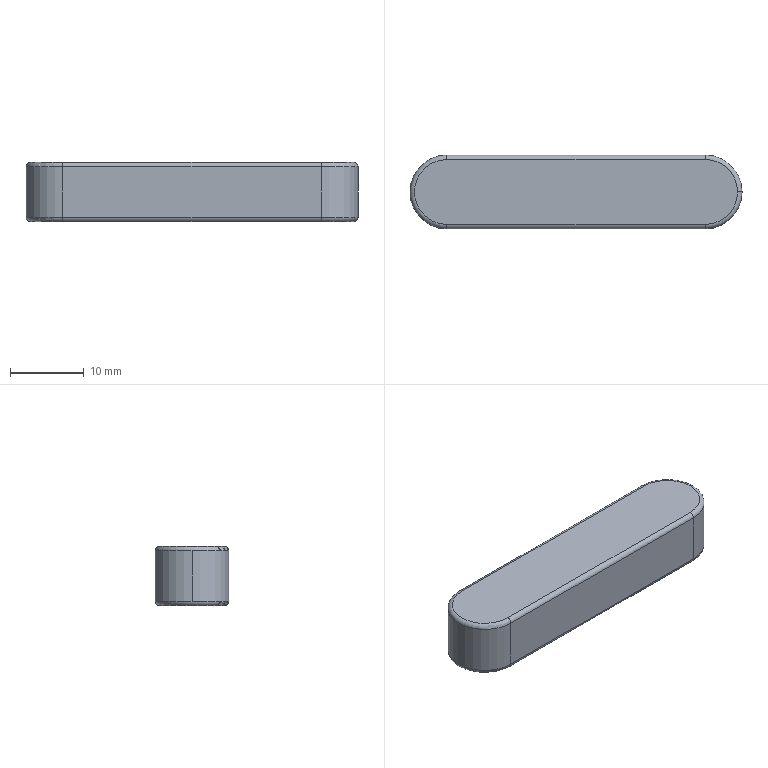Part | SolidWorks | features Extrusion 1, Fillet 1 | 1 solid | 17 faces | box 45 x 10 x 8 mm | volume 3413 mm3 | cylinder 7 | torus 6 | plane 4 | commonest cylinder face diameters 1.2 x4 10 x3
STEP:
#1=CARTESIAN_POINT('',(21.9,0.,0.));
#2=VERTEX_POINT('',#1);
#3=CARTESIAN_POINT('',(17.5,-4.4,0.));
#4=VERTEX_POINT('',#3);
#5=CARTESIAN_POINT('',(17.5,0.,0.));
#6=DIRECTION('',(0.,0.,-1.));
#7=DIRECTION('',(1.,0.,0.));
#8=AXIS2_PLACEMENT_3D('',#5,#6,#7);
#9=CIRCLE('',#8,4.4);
#10=EDGE_CURVE('',#2,#4,#9,.T.);
#11=ORIENTED_EDGE('',*,*,#10,.F.);
#12=CARTESIAN_POINT('',(22.5,0.,0.6));
#13=VERTEX_POINT('',#12);
#14=CARTESIAN_POINT('',(21.9,0.,0.6));
#15=DIRECTION('',(0.,-1.,0.));
#16=DIRECTION('',(0.,0.,-1.));
#17=AXIS2_PLACEMENT_3D('',#14,#15,#16);
#18=CIRCLE('',#17,0.6);
#19=EDGE_CURVE('',#2,#13,#18,.T.);
#20=ORIENTED_EDGE('',*,*,#19,.T.);
#21=CARTESIAN_POINT('',(17.5,-5.,0.6));
#22=VERTEX_POINT('',#21);
#23=CARTESIAN_POINT('',(17.5,0.,0.6));
#24=DIRECTION('',(0.,0.,1.));
#25=DIRECTION('',(1.,0.,0.));
#26=AXIS2_PLACEMENT_3D('',#23,#24,#25);
#27=CIRCLE('',#26,5.);
#28=EDGE_CURVE('',#22,#13,#27,.T.);
#29=ORIENTED_EDGE('',*,*,#28,.F.);
#30=CARTESIAN_POINT('',(17.5,-4.4,0.6));
#31=DIRECTION('',(1.,0.,0.));
#32=DIRECTION('',(0.,0.,-1.));
#33=AXIS2_PLACEMENT_3D('',#30,#31,#32);
#34=CIRCLE('',#33,0.6);
#35=EDGE_CURVE('',#22,#4,#34,.T.);
#36=ORIENTED_EDGE('',*,*,#35,.T.);
#37=EDGE_LOOP('',(#11,#20,#29,#36));
#38=FACE_OUTER_BOUND('',#37,.T.);
#39=CARTESIAN_POINT('',(17.5,0.,0.6));
#40=DIRECTION('',(0.,0.,1.));
#41=DIRECTION('',(1.,0.,0.));
#42=AXIS2_PLACEMENT_3D('',#39,#40,#41);
#43=TOROIDAL_SURFACE('',#42,4.4,0.6);
#44=ADVANCED_FACE('',(#38),#43,.T.);
#45=CARTESIAN_POINT('',(22.5,0.,7.4));
#46=VERTEX_POINT('',#45);
#47=CARTESIAN_POINT('',(17.5,-5.,7.4));
#48=VERTEX_POINT('',#47);
#49=CARTESIAN_POINT('',(17.5,0.,7.4));
#50=DIRECTION('',(0.,0.,-1.));
#51=DIRECTION('',(1.,0.,0.));
#52=AXIS2_PLACEMENT_3D('',#49,#50,#51);
#53=CIRCLE('',#52,5.);
#54=EDGE_CURVE('',#46,#48,#53,.T.);
#55=ORIENTED_EDGE('',*,*,#54,.F.);
#56=CARTESIAN_POINT('',(21.9,0.,8.));
#57=VERTEX_POINT('',#56);
#58=CARTESIAN_POINT('',(21.9,0.,7.4));
#59=DIRECTION('',(0.,-1.,0.));
#60=DIRECTION('',(0.,0.,-1.));
#61=AXIS2_PLACEMENT_3D('',#58,#59,#60);
#62=CIRCLE('',#61,0.6);
#63=EDGE_CURVE('',#46,#57,#62,.T.);
#64=ORIENTED_EDGE('',*,*,#63,.T.);
#65=CARTESIAN_POINT('',(17.5,-4.4,8.));
#66=VERTEX_POINT('',#65);
#67=CARTESIAN_POINT('',(17.5,0.,8.));
#68=DIRECTION('',(0.,0.,1.));
#69=DIRECTION('',(1.,0.,0.));
#70=AXIS2_PLACEMENT_3D('',#67,#68,#69);
#71=CIRCLE('',#70,4.4);
#72=EDGE_CURVE('',#66,#57,#71,.T.);
#73=ORIENTED_EDGE('',*,*,#72,.F.);
#74=CARTESIAN_POINT('',(17.5,-4.4,7.4));
#75=DIRECTION('',(1.,0.,0.));
#76=DIRECTION('',(0.,0.,-1.));
#77=AXIS2_PLACEMENT_3D('',#74,#75,#76);
#78=CIRCLE('',#77,0.6);
#79=EDGE_CURVE('',#66,#48,#78,.T.);
#80=ORIENTED_EDGE('',*,*,#79,.T.);
#81=EDGE_LOOP('',(#55,#64,#73,#80));
#82=FACE_OUTER_BOUND('',#81,.T.);
#83=CARTESIAN_POINT('',(17.5,0.,7.4));
#84=DIRECTION('',(0.,0.,1.));
#85=DIRECTION('',(1.,0.,0.));
#86=AXIS2_PLACEMENT_3D('',#83,#84,#85);
#87=TOROIDAL_SURFACE('',#86,4.4,0.6);
#88=ADVANCED_FACE('',(#82),#87,.T.);
#89=CARTESIAN_POINT('',(-17.5,-5.,7.4));
#90=VERTEX_POINT('',#89);
#91=CARTESIAN_POINT('',(-22.5,0.,7.4));
#92=VERTEX_POINT('',#91);
#93=CARTESIAN_POINT('',(-17.5,0.,7.4));
#94=DIRECTION('',(0.,0.,-1.));
#95=DIRECTION('',(1.,0.,0.));
#96=AXIS2_PLACEMENT_3D('',#93,#94,#95);
#97=CIRCLE('',#96,5.);
#98=EDGE_CURVE('',#90,#92,#97,.T.);
#99=ORIENTED_EDGE('',*,*,#98,.T.);
#100=CARTESIAN_POINT('',(-22.5,0.,0.6));
#101=VERTEX_POINT('',#100);
#102=CARTESIAN_POINT('',(-22.5,0.,8.));
#103=DIRECTION('',(0.,0.,-1.));
#104=VECTOR('',#103,1000.);
#105=LINE('',#102,#104);
#106=EDGE_CURVE('',#92,#101,#105,.T.);
#107=ORIENTED_EDGE('',*,*,#106,.T.);
#108=CARTESIAN_POINT('',(-17.5,-5.,0.6));
#109=VERTEX_POINT('',#108);
#110=CARTESIAN_POINT('',(-17.5,0.,0.6));
#111=DIRECTION('',(0.,0.,1.));
#112=DIRECTION('',(1.,0.,0.));
#113=AXIS2_PLACEMENT_3D('',#110,#111,#112);
#114=CIRCLE('',#113,5.);
#115=EDGE_CURVE('',#101,#109,#114,.T.);
#116=ORIENTED_EDGE('',*,*,#115,.T.);
#117=CARTESIAN_POINT('',(-17.5,-5.,8.));
#118=DIRECTION('',(0.,0.,-1.));
#119=VECTOR('',#118,1000.);
#120=LINE('',#117,#119);
#121=EDGE_CURVE('',#90,#109,#120,.T.);
#122=ORIENTED_EDGE('',*,*,#121,.F.);
#123=EDGE_LOOP('',(#99,#107,#116,#122));
#124=FACE_OUTER_BOUND('',#123,.T.);
#125=CARTESIAN_POINT('',(-17.5,0.,8.));
#126=DIRECTION('',(0.,0.,-1.));
#127=DIRECTION('',(-1.,0.,0.));
#128=AXIS2_PLACEMENT_3D('',#125,#126,#127);
#129=CYLINDRICAL_SURFACE('',#128,5.);
#130=ADVANCED_FACE('',(#124),#129,.T.);
#131=ORIENTED_EDGE('',*,*,#106,.F.);
#132=CARTESIAN_POINT('',(-17.5,5.,7.4));
#133=VERTEX_POINT('',#132);
#134=CARTESIAN_POINT('',(-17.5,0.,7.4));
#135=DIRECTION('',(0.,0.,-1.));
#136=DIRECTION('',(1.,0.,0.));
#137=AXIS2_PLACEMENT_3D('',#134,#135,#136);
#138=CIRCLE('',#137,5.);
#139=EDGE_CURVE('',#92,#133,#138,.T.);
#140=ORIENTED_EDGE('',*,*,#139,.T.);
#141=CARTESIAN_POINT('',(-17.5,5.,0.6));
#142=VERTEX_POINT('',#141);
#143=CARTESIAN_POINT('',(-17.5,5.,8.));
#144=DIRECTION('',(0.,0.,-1.));
#145=VECTOR('',#144,1000.);
#146=LINE('',#143,#145);
#147=EDGE_CURVE('',#133,#142,#146,.T.);
#148=ORIENTED_EDGE('',*,*,#147,.T.);
#149=CARTESIAN_POINT('',(-17.5,0.,0.6));
#150=DIRECTION('',(0.,0.,1.));
#151=DIRECTION('',(1.,0.,0.));
#152=AXIS2_PLACEMENT_3D('',#149,#150,#151);
#153=CIRCLE('',#152,5.);
#154=EDGE_CURVE('',#142,#101,#153,.T.);
#155=ORIENTED_EDGE('',*,*,#154,.T.);
#156=EDGE_LOOP('',(#131,#140,#148,#155));
#157=FACE_OUTER_BOUND('',#156,.T.);
#158=CARTESIAN_POINT('',(-17.5,0.,8.));
#159=DIRECTION('',(0.,0.,-1.));
#160=DIRECTION('',(-1.,0.,0.));
#161=AXIS2_PLACEMENT_3D('',#158,#159,#160);
#162=CYLINDRICAL_SURFACE('',#161,5.);
#163=ADVANCED_FACE('',(#157),#162,.T.);
#164=CARTESIAN_POINT('',(17.5,-5.,8.));
#165=DIRECTION('',(0.,0.,-1.));
#166=VECTOR('',#165,1000.);
#167=LINE('',#164,#166);
#168=EDGE_CURVE('',#48,#22,#167,.T.);
#169=ORIENTED_EDGE('',*,*,#168,.F.);
#170=CARTESIAN_POINT('',(-17.5,-5.,7.4));
#171=DIRECTION('',(-1.,0.,0.));
#172=VECTOR('',#171,1000.);
#173=LINE('',#170,#172);
#174=EDGE_CURVE('',#48,#90,#173,.T.);
#175=ORIENTED_EDGE('',*,*,#174,.T.);
#176=ORIENTED_EDGE('',*,*,#121,.T.);
#177=CARTESIAN_POINT('',(-17.5,-5.,0.6));
#178=DIRECTION('',(1.,0.,0.));
#179=VECTOR('',#178,1000.);
#180=LINE('',#177,#179);
#181=EDGE_CURVE('',#109,#22,#180,.T.);
#182=ORIENTED_EDGE('',*,*,#181,.T.);
#183=EDGE_LOOP('',(#169,#175,#176,#182));
#184=FACE_OUTER_BOUND('',#183,.T.);
#185=CARTESIAN_POINT('',(-17.5,-5.,8.));
#186=DIRECTION('',(0.,1.,0.));
#187=DIRECTION('',(-1.,0.,0.));
#188=AXIS2_PLACEMENT_3D('',#185,#186,#187);
#189=PLANE('',#188);
#190=ADVANCED_FACE('',(#184),#189,.F.);
#191=CARTESIAN_POINT('',(17.5,5.,7.4));
#192=VERTEX_POINT('',#191);
#193=CARTESIAN_POINT('',(17.5,5.,0.6));
#194=VERTEX_POINT('',#193);
#195=CARTESIAN_POINT('',(17.5,5.,8.));
#196=DIRECTION('',(0.,0.,-1.));
#197=VECTOR('',#196,1000.);
#198=LINE('',#195,#197);
#199=EDGE_CURVE('',#192,#194,#198,.T.);
#200=ORIENTED_EDGE('',*,*,#199,.F.);
#201=CARTESIAN_POINT('',(17.5,0.,7.4));
#202=DIRECTION('',(0.,0.,-1.));
#203=DIRECTION('',(1.,0.,0.));
#204=AXIS2_PLACEMENT_3D('',#201,#202,#203);
#205=CIRCLE('',#204,5.);
#206=EDGE_CURVE('',#192,#46,#205,.T.);
#207=ORIENTED_EDGE('',*,*,#206,.T.);
#208=ORIENTED_EDGE('',*,*,#54,.T.);
#209=ORIENTED_EDGE('',*,*,#168,.T.);
#210=ORIENTED_EDGE('',*,*,#28,.T.);
#211=CARTESIAN_POINT('',(17.5,0.,0.6));
#212=DIRECTION('',(0.,0.,1.));
#213=DIRECTION('',(1.,0.,0.));
#214=AXIS2_PLACEMENT_3D('',#211,#212,#213);
#215=CIRCLE('',#214,5.);
#216=EDGE_CURVE('',#13,#194,#215,.T.);
#217=ORIENTED_EDGE('',*,*,#216,.T.);
#218=EDGE_LOOP('',(#200,#207,#208,#209,#210,#217));
#219=FACE_OUTER_BOUND('',#218,.T.);
#220=CARTESIAN_POINT('',(17.5,0.,8.));
#221=DIRECTION('',(0.,0.,-1.));
#222=DIRECTION('',(-1.,0.,0.));
#223=AXIS2_PLACEMENT_3D('',#220,#221,#222);
#224=CYLINDRICAL_SURFACE('',#223,5.);
#225=ADVANCED_FACE('',(#219),#224,.T.);
#226=ORIENTED_EDGE('',*,*,#147,.F.);
#227=CARTESIAN_POINT('',(17.5,5.,7.4));
#228=DIRECTION('',(1.,0.,0.));
#229=VECTOR('',#228,1000.);
#230=LINE('',#227,#229);
#231=EDGE_CURVE('',#133,#192,#230,.T.);
#232=ORIENTED_EDGE('',*,*,#231,.T.);
#233=ORIENTED_EDGE('',*,*,#199,.T.);
#234=CARTESIAN_POINT('',(-17.5,5.,0.6));
#235=DIRECTION('',(-1.,0.,0.));
#236=VECTOR('',#235,1000.);
#237=LINE('',#234,#236);
#238=EDGE_CURVE('',#194,#142,#237,.T.);
#239=ORIENTED_EDGE('',*,*,#238,.T.);
#240=EDGE_LOOP('',(#226,#232,#233,#239));
#241=FACE_OUTER_BOUND('',#240,.T.);
#242=CARTESIAN_POINT('',(-17.5,5.,8.));
#243=DIRECTION('',(0.,-1.,0.));
#244=DIRECTION('',(1.,0.,0.));
#245=AXIS2_PLACEMENT_3D('',#242,#243,#244);
#246=PLANE('',#245);
#247=ADVANCED_FACE('',(#241),#246,.F.);
#248=CARTESIAN_POINT('',(-17.5,-4.4,8.));
#249=VERTEX_POINT('',#248);
#250=CARTESIAN_POINT('',(17.5,-4.4,8.));
#251=DIRECTION('',(1.,0.,0.));
#252=VECTOR('',#251,1000.);
#253=LINE('',#250,#252);
#254=EDGE_CURVE('',#249,#66,#253,.T.);
#255=ORIENTED_EDGE('',*,*,#254,.T.);
#256=ORIENTED_EDGE('',*,*,#72,.T.);
#257=CARTESIAN_POINT('',(17.5,4.4,8.));
#258=VERTEX_POINT('',#257);
#259=CARTESIAN_POINT('',(17.5,0.,8.));
#260=DIRECTION('',(0.,0.,1.));
#261=DIRECTION('',(1.,0.,0.));
#262=AXIS2_PLACEMENT_3D('',#259,#260,#261);
#263=CIRCLE('',#262,4.4);
#264=EDGE_CURVE('',#57,#258,#263,.T.);
#265=ORIENTED_EDGE('',*,*,#264,.T.);
#266=CARTESIAN_POINT('',(-17.5,4.4,8.));
#267=VERTEX_POINT('',#266);
#268=CARTESIAN_POINT('',(-17.5,4.4,8.));
#269=DIRECTION('',(-1.,0.,0.));
#270=VECTOR('',#269,1000.);
#271=LINE('',#268,#270);
#272=EDGE_CURVE('',#258,#267,#271,.T.);
#273=ORIENTED_EDGE('',*,*,#272,.T.);
#274=CARTESIAN_POINT('',(-17.5,0.,8.));
#275=DIRECTION('',(0.,0.,1.));
#276=DIRECTION('',(1.,0.,0.));
#277=AXIS2_PLACEMENT_3D('',#274,#275,#276);
#278=CIRCLE('',#277,4.4);
#279=EDGE_CURVE('',#267,#249,#278,.T.);
#280=ORIENTED_EDGE('',*,*,#279,.T.);
#281=EDGE_LOOP('',(#255,#256,#265,#273,#280));
#282=FACE_OUTER_BOUND('',#281,.T.);
#283=CARTESIAN_POINT('',(-17.5,0.,8.));
#284=DIRECTION('',(0.,0.,1.));
#285=DIRECTION('',(1.,0.,0.));
#286=AXIS2_PLACEMENT_3D('',#283,#284,#285);
#287=PLANE('',#286);
#288=ADVANCED_FACE('',(#282),#287,.T.);
#289=CARTESIAN_POINT('',(-17.5,4.4,0.));
#290=VERTEX_POINT('',#289);
#291=CARTESIAN_POINT('',(17.5,4.4,0.));
#292=VERTEX_POINT('',#291);
#293=CARTESIAN_POINT('',(-17.5,4.4,0.));
#294=DIRECTION('',(1.,0.,0.));
#295=VECTOR('',#294,1000.);
#296=LINE('',#293,#295);
#297=EDGE_CURVE('',#290,#292,#296,.T.);
#298=ORIENTED_EDGE('',*,*,#297,.T.);
#299=CARTESIAN_POINT('',(17.5,0.,0.));
#300=DIRECTION('',(0.,0.,-1.));
#301=DIRECTION('',(1.,0.,0.));
#302=AXIS2_PLACEMENT_3D('',#299,#300,#301);
#303=CIRCLE('',#302,4.4);
#304=EDGE_CURVE('',#292,#2,#303,.T.);
#305=ORIENTED_EDGE('',*,*,#304,.T.);
#306=ORIENTED_EDGE('',*,*,#10,.T.);
#307=CARTESIAN_POINT('',(-17.5,-4.4,0.));
#308=VERTEX_POINT('',#307);
#309=CARTESIAN_POINT('',(-17.5,-4.4,0.));
#310=DIRECTION('',(-1.,0.,0.));
#311=VECTOR('',#310,1000.);
#312=LINE('',#309,#311);
#313=EDGE_CURVE('',#4,#308,#312,.T.);
#314=ORIENTED_EDGE('',*,*,#313,.T.);
#315=CARTESIAN_POINT('',(-17.5,0.,0.));
#316=DIRECTION('',(0.,0.,-1.));
#317=DIRECTION('',(1.,0.,0.));
#318=AXIS2_PLACEMENT_3D('',#315,#316,#317);
#319=CIRCLE('',#318,4.4);
#320=EDGE_CURVE('',#308,#290,#319,.T.);
#321=ORIENTED_EDGE('',*,*,#320,.T.);
#322=EDGE_LOOP('',(#298,#305,#306,#314,#321));
#323=FACE_OUTER_BOUND('',#322,.T.);
#324=CARTESIAN_POINT('',(-17.5,0.,0.));
#325=DIRECTION('',(0.,0.,1.));
#326=DIRECTION('',(1.,0.,0.));
#327=AXIS2_PLACEMENT_3D('',#324,#325,#326);
#328=PLANE('',#327);
#329=ADVANCED_FACE('',(#323),#328,.F.);
#330=CARTESIAN_POINT('',(-17.5,4.4,7.4));
#331=DIRECTION('',(1.,0.,0.));
#332=DIRECTION('',(0.,0.,-1.));
#333=AXIS2_PLACEMENT_3D('',#330,#331,#332);
#334=CIRCLE('',#333,0.6);
#335=EDGE_CURVE('',#133,#267,#334,.T.);
#336=ORIENTED_EDGE('',*,*,#335,.F.);
#337=ORIENTED_EDGE('',*,*,#139,.F.);
#338=ORIENTED_EDGE('',*,*,#98,.F.);
#339=CARTESIAN_POINT('',(-17.5,-4.4,7.4));
#340=DIRECTION('',(1.,0.,0.));
#341=DIRECTION('',(0.,0.,-1.));
#342=AXIS2_PLACEMENT_3D('',#339,#340,#341);
#343=CIRCLE('',#342,0.6);
#344=EDGE_CURVE('',#249,#90,#343,.T.);
#345=ORIENTED_EDGE('',*,*,#344,.F.);
#346=ORIENTED_EDGE('',*,*,#279,.F.);
#347=EDGE_LOOP('',(#336,#337,#338,#345,#346));
#348=FACE_OUTER_BOUND('',#347,.T.);
#349=CARTESIAN_POINT('',(-17.5,0.,7.4));
#350=DIRECTION('',(0.,0.,1.));
#351=DIRECTION('',(1.,0.,0.));
#352=AXIS2_PLACEMENT_3D('',#349,#350,#351);
#353=TOROIDAL_SURFACE('',#352,4.4,0.6);
#354=ADVANCED_FACE('',(#348),#353,.T.);
#355=ORIENTED_EDGE('',*,*,#344,.T.);
#356=ORIENTED_EDGE('',*,*,#174,.F.);
#357=ORIENTED_EDGE('',*,*,#79,.F.);
#358=ORIENTED_EDGE('',*,*,#254,.F.);
#359=EDGE_LOOP('',(#355,#356,#357,#358));
#360=FACE_OUTER_BOUND('',#359,.T.);
#361=CARTESIAN_POINT('',(-17.5,-4.4,7.4));
#362=DIRECTION('',(-1.,0.,0.));
#363=DIRECTION('',(0.,-1.,0.));
#364=AXIS2_PLACEMENT_3D('',#361,#362,#363);
#365=CYLINDRICAL_SURFACE('',#364,0.6);
#366=ADVANCED_FACE('',(#360),#365,.T.);
#367=ORIENTED_EDGE('',*,*,#335,.T.);
#368=ORIENTED_EDGE('',*,*,#272,.F.);
#369=CARTESIAN_POINT('',(17.5,4.4,7.4));
#370=DIRECTION('',(1.,0.,0.));
#371=DIRECTION('',(0.,0.,-1.));
#372=AXIS2_PLACEMENT_3D('',#369,#370,#371);
#373=CIRCLE('',#372,0.6);
#374=EDGE_CURVE('',#192,#258,#373,.T.);
#375=ORIENTED_EDGE('',*,*,#374,.F.);
#376=ORIENTED_EDGE('',*,*,#231,.F.);
#377=EDGE_LOOP('',(#367,#368,#375,#376));
#378=FACE_OUTER_BOUND('',#377,.T.);
#379=CARTESIAN_POINT('',(-17.5,4.4,7.4));
#380=DIRECTION('',(1.,0.,0.));
#381=DIRECTION('',(0.,1.,0.));
#382=AXIS2_PLACEMENT_3D('',#379,#380,#381);
#383=CYLINDRICAL_SURFACE('',#382,0.6);
#384=ADVANCED_FACE('',(#378),#383,.T.);
#385=ORIENTED_EDGE('',*,*,#63,.F.);
#386=ORIENTED_EDGE('',*,*,#206,.F.);
#387=ORIENTED_EDGE('',*,*,#374,.T.);
#388=ORIENTED_EDGE('',*,*,#264,.F.);
#389=EDGE_LOOP('',(#385,#386,#387,#388));
#390=FACE_OUTER_BOUND('',#389,.T.);
#391=CARTESIAN_POINT('',(17.5,0.,7.4));
#392=DIRECTION('',(0.,0.,1.));
#393=DIRECTION('',(1.,0.,0.));
#394=AXIS2_PLACEMENT_3D('',#391,#392,#393);
#395=TOROIDAL_SURFACE('',#394,4.4,0.6);
#396=ADVANCED_FACE('',(#390),#395,.T.);
#397=CARTESIAN_POINT('',(-17.5,4.4,0.6));
#398=DIRECTION('',(1.,0.,0.));
#399=DIRECTION('',(0.,0.,-1.));
#400=AXIS2_PLACEMENT_3D('',#397,#398,#399);
#401=CIRCLE('',#400,0.6);
#402=EDGE_CURVE('',#290,#142,#401,.T.);
#403=ORIENTED_EDGE('',*,*,#402,.F.);
#404=ORIENTED_EDGE('',*,*,#320,.F.);
#405=CARTESIAN_POINT('',(-17.5,-4.4,0.6));
#406=DIRECTION('',(1.,0.,0.));
#407=DIRECTION('',(0.,0.,-1.));
#408=AXIS2_PLACEMENT_3D('',#405,#406,#407);
#409=CIRCLE('',#408,0.6);
#410=EDGE_CURVE('',#109,#308,#409,.T.);
#411=ORIENTED_EDGE('',*,*,#410,.F.);
#412=ORIENTED_EDGE('',*,*,#115,.F.);
#413=ORIENTED_EDGE('',*,*,#154,.F.);
#414=EDGE_LOOP('',(#403,#404,#411,#412,#413));
#415=FACE_OUTER_BOUND('',#414,.T.);
#416=CARTESIAN_POINT('',(-17.5,0.,0.6));
#417=DIRECTION('',(0.,0.,1.));
#418=DIRECTION('',(1.,0.,0.));
#419=AXIS2_PLACEMENT_3D('',#416,#417,#418);
#420=TOROIDAL_SURFACE('',#419,4.4,0.6);
#421=ADVANCED_FACE('',(#415),#420,.T.);
#422=ORIENTED_EDGE('',*,*,#410,.T.);
#423=ORIENTED_EDGE('',*,*,#313,.F.);
#424=ORIENTED_EDGE('',*,*,#35,.F.);
#425=ORIENTED_EDGE('',*,*,#181,.F.);
#426=EDGE_LOOP('',(#422,#423,#424,#425));
#427=FACE_OUTER_BOUND('',#426,.T.);
#428=CARTESIAN_POINT('',(-17.5,-4.4,0.6));
#429=DIRECTION('',(1.,0.,0.));
#430=DIRECTION('',(0.,1.,0.));
#431=AXIS2_PLACEMENT_3D('',#428,#429,#430);
#432=CYLINDRICAL_SURFACE('',#431,0.6);
#433=ADVANCED_FACE('',(#427),#432,.T.);
#434=ORIENTED_EDGE('',*,*,#402,.T.);
#435=ORIENTED_EDGE('',*,*,#238,.F.);
#436=CARTESIAN_POINT('',(17.5,4.4,0.6));
#437=DIRECTION('',(1.,0.,0.));
#438=DIRECTION('',(0.,0.,-1.));
#439=AXIS2_PLACEMENT_3D('',#436,#437,#438);
#440=CIRCLE('',#439,0.6);
#441=EDGE_CURVE('',#292,#194,#440,.T.);
#442=ORIENTED_EDGE('',*,*,#441,.F.);
#443=ORIENTED_EDGE('',*,*,#297,.F.);
#444=EDGE_LOOP('',(#434,#435,#442,#443));
#445=FACE_OUTER_BOUND('',#444,.T.);
#446=CARTESIAN_POINT('',(-17.5,4.4,0.6));
#447=DIRECTION('',(-1.,0.,0.));
#448=DIRECTION('',(0.,-1.,0.));
#449=AXIS2_PLACEMENT_3D('',#446,#447,#448);
#450=CYLINDRICAL_SURFACE('',#449,0.6);
#451=ADVANCED_FACE('',(#445),#450,.T.);
#452=ORIENTED_EDGE('',*,*,#19,.F.);
#453=ORIENTED_EDGE('',*,*,#304,.F.);
#454=ORIENTED_EDGE('',*,*,#441,.T.);
#455=ORIENTED_EDGE('',*,*,#216,.F.);
#456=EDGE_LOOP('',(#452,#453,#454,#455));
#457=FACE_OUTER_BOUND('',#456,.T.);
#458=CARTESIAN_POINT('',(17.5,0.,0.6));
#459=DIRECTION('',(0.,0.,1.));
#460=DIRECTION('',(1.,0.,0.));
#461=AXIS2_PLACEMENT_3D('',#458,#459,#460);
#462=TOROIDAL_SURFACE('',#461,4.4,0.6);
#463=ADVANCED_FACE('',(#457),#462,.T.);
#464=CLOSED_SHELL('',(#44,#88,#130,#163,#190,#225,#247,#288,#329,#354,#366,#384,#396,#421,#433,#451,#463));
#465=MANIFOLD_SOLID_BREP('',#464);
#466=CARTESIAN_POINT('',(0.,0.,0.));
#467=DIRECTION('',(0.,0.,1.));
#468=DIRECTION('',(1.,0.,0.));
#469=AXIS2_PLACEMENT_3D('',#466,#467,#468);
#470=(LENGTH_UNIT()NAMED_UNIT(*)SI_UNIT(.MILLI.,.METRE.));
#471=UNCERTAINTY_MEASURE_WITH_UNIT(LENGTH_MEASURE(0.00001),#470,'','');
#472=(NAMED_UNIT(*)PLANE_ANGLE_UNIT()SI_UNIT($,.RADIAN.));
#473=(NAMED_UNIT(*)SI_UNIT($,.STERADIAN.)SOLID_ANGLE_UNIT());
#474=(GEOMETRIC_REPRESENTATION_CONTEXT(3)GLOBAL_UNCERTAINTY_ASSIGNED_CONTEXT((#471))GLOBAL_UNIT_ASSIGNED_CONTEXT((#470,#472,#473))REPRESENTATION_CONTEXT('',''));
#475=ADVANCED_BREP_SHAPE_REPRESENTATION('',(#465,#469),#474);